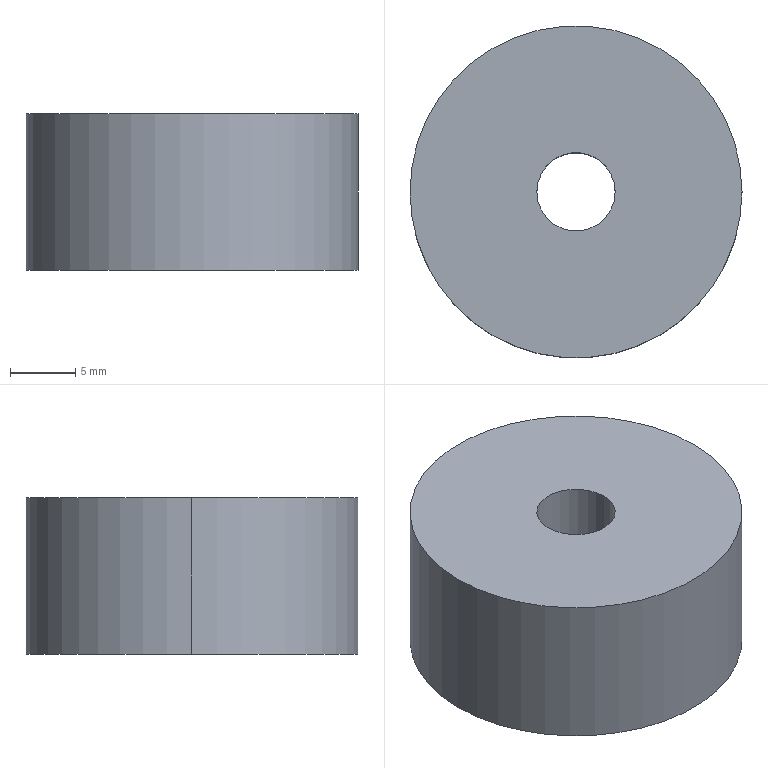Part | SolidWorks | features Extrusion 1 | 1 solid | 6 faces | box 25.4 x 25.4 x 12 mm | volume 5741 mm3 | cylinder 4 | plane 2 | commonest cylinder face diameters 6 x2 25.4 x2
STEP:
#1=CARTESIAN_POINT('',(-3.,0.,12.));
#2=VERTEX_POINT('',#1);
#3=CARTESIAN_POINT('',(3.,0.,12.));
#4=VERTEX_POINT('',#3);
#5=CARTESIAN_POINT('',(0.,0.,12.));
#6=DIRECTION('',(0.,0.,1.));
#7=DIRECTION('',(1.,0.,0.));
#8=AXIS2_PLACEMENT_3D('',#5,#6,#7);
#9=CIRCLE('',#8,3.);
#10=EDGE_CURVE('',#2,#4,#9,.T.);
#11=ORIENTED_EDGE('',*,*,#10,.T.);
#12=CARTESIAN_POINT('',(3.,0.,0.));
#13=VERTEX_POINT('',#12);
#14=CARTESIAN_POINT('',(3.,0.,12.));
#15=DIRECTION('',(0.,0.,-1.));
#16=VECTOR('',#15,1000.);
#17=LINE('',#14,#16);
#18=EDGE_CURVE('',#4,#13,#17,.T.);
#19=ORIENTED_EDGE('',*,*,#18,.T.);
#20=CARTESIAN_POINT('',(-3.,0.,0.));
#21=VERTEX_POINT('',#20);
#22=CARTESIAN_POINT('',(0.,0.,0.));
#23=DIRECTION('',(0.,0.,1.));
#24=DIRECTION('',(1.,0.,0.));
#25=AXIS2_PLACEMENT_3D('',#22,#23,#24);
#26=CIRCLE('',#25,3.);
#27=EDGE_CURVE('',#21,#13,#26,.T.);
#28=ORIENTED_EDGE('',*,*,#27,.F.);
#29=CARTESIAN_POINT('',(-3.,0.,12.));
#30=DIRECTION('',(0.,0.,-1.));
#31=VECTOR('',#30,1000.);
#32=LINE('',#29,#31);
#33=EDGE_CURVE('',#2,#21,#32,.T.);
#34=ORIENTED_EDGE('',*,*,#33,.F.);
#35=EDGE_LOOP('',(#11,#19,#28,#34));
#36=FACE_OUTER_BOUND('',#35,.T.);
#37=CARTESIAN_POINT('',(0.,0.,12.));
#38=DIRECTION('',(0.,0.,-1.));
#39=DIRECTION('',(-1.,0.,0.));
#40=AXIS2_PLACEMENT_3D('',#37,#38,#39);
#41=CYLINDRICAL_SURFACE('',#40,3.);
#42=ADVANCED_FACE('',(#36),#41,.F.);
#43=CARTESIAN_POINT('',(12.7,0.,12.));
#44=VERTEX_POINT('',#43);
#45=CARTESIAN_POINT('',(-12.7,0.,12.));
#46=VERTEX_POINT('',#45);
#47=CARTESIAN_POINT('',(0.,0.,12.));
#48=DIRECTION('',(0.,0.,1.));
#49=DIRECTION('',(1.,0.,0.));
#50=AXIS2_PLACEMENT_3D('',#47,#48,#49);
#51=CIRCLE('',#50,12.7);
#52=EDGE_CURVE('',#44,#46,#51,.T.);
#53=ORIENTED_EDGE('',*,*,#52,.F.);
#54=CARTESIAN_POINT('',(12.7,0.,0.));
#55=VERTEX_POINT('',#54);
#56=CARTESIAN_POINT('',(12.7,0.,12.));
#57=DIRECTION('',(0.,0.,-1.));
#58=VECTOR('',#57,1000.);
#59=LINE('',#56,#58);
#60=EDGE_CURVE('',#44,#55,#59,.T.);
#61=ORIENTED_EDGE('',*,*,#60,.T.);
#62=CARTESIAN_POINT('',(-12.7,0.,0.));
#63=VERTEX_POINT('',#62);
#64=CARTESIAN_POINT('',(0.,0.,0.));
#65=DIRECTION('',(0.,0.,1.));
#66=DIRECTION('',(1.,0.,0.));
#67=AXIS2_PLACEMENT_3D('',#64,#65,#66);
#68=CIRCLE('',#67,12.7);
#69=EDGE_CURVE('',#55,#63,#68,.T.);
#70=ORIENTED_EDGE('',*,*,#69,.T.);
#71=CARTESIAN_POINT('',(-12.7,0.,12.));
#72=DIRECTION('',(0.,0.,-1.));
#73=VECTOR('',#72,1000.);
#74=LINE('',#71,#73);
#75=EDGE_CURVE('',#46,#63,#74,.T.);
#76=ORIENTED_EDGE('',*,*,#75,.F.);
#77=EDGE_LOOP('',(#53,#61,#70,#76));
#78=FACE_OUTER_BOUND('',#77,.T.);
#79=CARTESIAN_POINT('',(0.,0.,12.));
#80=DIRECTION('',(0.,0.,-1.));
#81=DIRECTION('',(-1.,0.,0.));
#82=AXIS2_PLACEMENT_3D('',#79,#80,#81);
#83=CYLINDRICAL_SURFACE('',#82,12.7);
#84=ADVANCED_FACE('',(#78),#83,.T.);
#85=CARTESIAN_POINT('',(0.,0.,12.));
#86=DIRECTION('',(0.,0.,1.));
#87=DIRECTION('',(1.,0.,0.));
#88=AXIS2_PLACEMENT_3D('',#85,#86,#87);
#89=CIRCLE('',#88,12.7);
#90=EDGE_CURVE('',#46,#44,#89,.T.);
#91=ORIENTED_EDGE('',*,*,#90,.T.);
#92=ORIENTED_EDGE('',*,*,#52,.T.);
#93=EDGE_LOOP('',(#91,#92));
#94=FACE_OUTER_BOUND('',#93,.T.);
#95=ORIENTED_EDGE('',*,*,#10,.F.);
#96=CARTESIAN_POINT('',(0.,0.,12.));
#97=DIRECTION('',(0.,0.,1.));
#98=DIRECTION('',(1.,0.,0.));
#99=AXIS2_PLACEMENT_3D('',#96,#97,#98);
#100=CIRCLE('',#99,3.);
#101=EDGE_CURVE('',#4,#2,#100,.T.);
#102=ORIENTED_EDGE('',*,*,#101,.F.);
#103=EDGE_LOOP('',(#95,#102));
#104=FACE_BOUND('',#103,.T.);
#105=CARTESIAN_POINT('',(0.,0.,12.));
#106=DIRECTION('',(0.,0.,1.));
#107=DIRECTION('',(1.,0.,0.));
#108=AXIS2_PLACEMENT_3D('',#105,#106,#107);
#109=PLANE('',#108);
#110=ADVANCED_FACE('',(#94,#104),#109,.T.);
#111=CARTESIAN_POINT('',(0.,0.,0.));
#112=DIRECTION('',(0.,0.,1.));
#113=DIRECTION('',(1.,0.,0.));
#114=AXIS2_PLACEMENT_3D('',#111,#112,#113);
#115=CIRCLE('',#114,12.7);
#116=EDGE_CURVE('',#63,#55,#115,.T.);
#117=ORIENTED_EDGE('',*,*,#116,.F.);
#118=ORIENTED_EDGE('',*,*,#69,.F.);
#119=EDGE_LOOP('',(#117,#118));
#120=FACE_OUTER_BOUND('',#119,.T.);
#121=ORIENTED_EDGE('',*,*,#27,.T.);
#122=CARTESIAN_POINT('',(0.,0.,0.));
#123=DIRECTION('',(0.,0.,1.));
#124=DIRECTION('',(1.,0.,0.));
#125=AXIS2_PLACEMENT_3D('',#122,#123,#124);
#126=CIRCLE('',#125,3.);
#127=EDGE_CURVE('',#13,#21,#126,.T.);
#128=ORIENTED_EDGE('',*,*,#127,.T.);
#129=EDGE_LOOP('',(#121,#128));
#130=FACE_BOUND('',#129,.T.);
#131=CARTESIAN_POINT('',(0.,0.,0.));
#132=DIRECTION('',(0.,0.,1.));
#133=DIRECTION('',(1.,0.,0.));
#134=AXIS2_PLACEMENT_3D('',#131,#132,#133);
#135=PLANE('',#134);
#136=ADVANCED_FACE('',(#120,#130),#135,.F.);
#137=ORIENTED_EDGE('',*,*,#60,.F.);
#138=ORIENTED_EDGE('',*,*,#90,.F.);
#139=ORIENTED_EDGE('',*,*,#75,.T.);
#140=ORIENTED_EDGE('',*,*,#116,.T.);
#141=EDGE_LOOP('',(#137,#138,#139,#140));
#142=FACE_OUTER_BOUND('',#141,.T.);
#143=CARTESIAN_POINT('',(0.,0.,12.));
#144=DIRECTION('',(0.,0.,-1.));
#145=DIRECTION('',(-1.,0.,0.));
#146=AXIS2_PLACEMENT_3D('',#143,#144,#145);
#147=CYLINDRICAL_SURFACE('',#146,12.7);
#148=ADVANCED_FACE('',(#142),#147,.T.);
#149=ORIENTED_EDGE('',*,*,#18,.F.);
#150=ORIENTED_EDGE('',*,*,#101,.T.);
#151=ORIENTED_EDGE('',*,*,#33,.T.);
#152=ORIENTED_EDGE('',*,*,#127,.F.);
#153=EDGE_LOOP('',(#149,#150,#151,#152));
#154=FACE_OUTER_BOUND('',#153,.T.);
#155=CARTESIAN_POINT('',(0.,0.,12.));
#156=DIRECTION('',(0.,0.,-1.));
#157=DIRECTION('',(-1.,0.,0.));
#158=AXIS2_PLACEMENT_3D('',#155,#156,#157);
#159=CYLINDRICAL_SURFACE('',#158,3.);
#160=ADVANCED_FACE('',(#154),#159,.F.);
#161=CLOSED_SHELL('',(#42,#84,#110,#136,#148,#160));
#162=MANIFOLD_SOLID_BREP('',#161);
#163=CARTESIAN_POINT('',(0.,0.,0.));
#164=DIRECTION('',(0.,0.,1.));
#165=DIRECTION('',(1.,0.,0.));
#166=AXIS2_PLACEMENT_3D('',#163,#164,#165);
#167=(LENGTH_UNIT()NAMED_UNIT(*)SI_UNIT(.MILLI.,.METRE.));
#168=UNCERTAINTY_MEASURE_WITH_UNIT(LENGTH_MEASURE(0.00001),#167,'','');
#169=(NAMED_UNIT(*)PLANE_ANGLE_UNIT()SI_UNIT($,.RADIAN.));
#170=(NAMED_UNIT(*)SI_UNIT($,.STERADIAN.)SOLID_ANGLE_UNIT());
#171=(GEOMETRIC_REPRESENTATION_CONTEXT(3)GLOBAL_UNCERTAINTY_ASSIGNED_CONTEXT((#168))GLOBAL_UNIT_ASSIGNED_CONTEXT((#167,#169,#170))REPRESENTATION_CONTEXT('',''));
#172=ADVANCED_BREP_SHAPE_REPRESENTATION('',(#162,#166),#171);